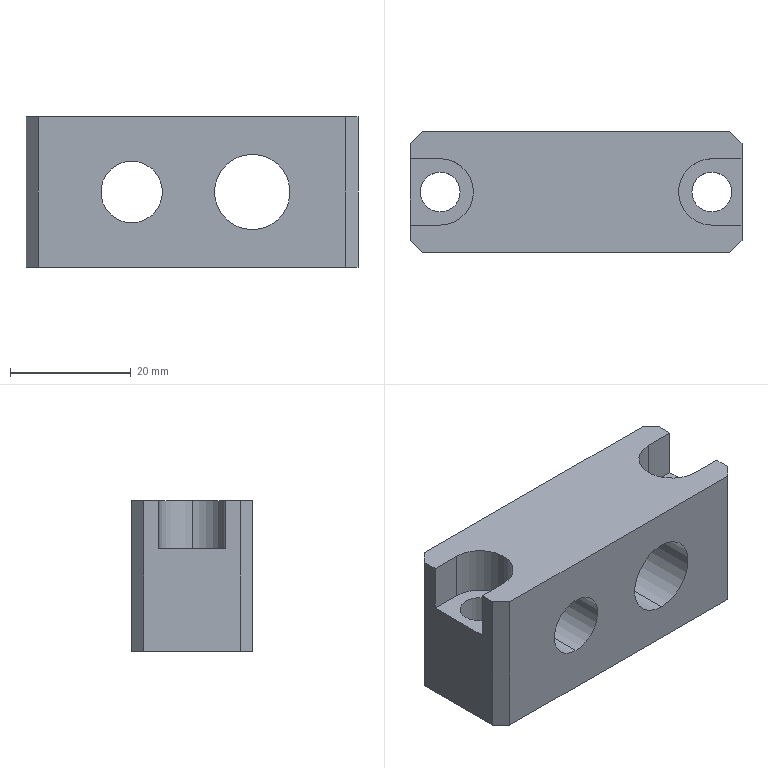Part | SolidWorks | features HoleWzd 3, Chamfer 1, Extrusion 1, ICE 1 | 1 solid | 27 faces | box 55 x 20 x 25 mm | volume 20408 mm3 | plane 16 | cylinder 11 | commonest cylinder face diameters 6.6 x4 11 x3 10.2 x2 12.5 x2
STEP:
#1=CARTESIAN_POINT('',(10.549,13.11,18.75));
#2=VERTEX_POINT('',#1);
#3=CARTESIAN_POINT('',(10.549,13.11,6.25));
#4=VERTEX_POINT('',#3);
#5=CARTESIAN_POINT('',(10.549,13.11,12.5));
#6=DIRECTION('',(0.,-1.,0.));
#7=DIRECTION('',(0.,0.,-1.));
#8=AXIS2_PLACEMENT_3D('',#5,#6,#7);
#9=CIRCLE('',#8,6.25);
#10=EDGE_CURVE('',#2,#4,#9,.T.);
#11=ORIENTED_EDGE('',*,*,#10,.F.);
#12=CARTESIAN_POINT('',(10.549,-6.89,18.75));
#13=VERTEX_POINT('',#12);
#14=CARTESIAN_POINT('',(10.549,-6.89,18.75));
#15=DIRECTION('',(0.,-1.,0.));
#16=VECTOR('',#15,1000.);
#17=LINE('',#14,#16);
#18=EDGE_CURVE('',#2,#13,#17,.T.);
#19=ORIENTED_EDGE('',*,*,#18,.T.);
#20=CARTESIAN_POINT('',(10.549,-6.89,6.25));
#21=VERTEX_POINT('',#20);
#22=CARTESIAN_POINT('',(10.549,-6.89,12.5));
#23=DIRECTION('',(0.,-1.,0.));
#24=DIRECTION('',(0.,0.,-1.));
#25=AXIS2_PLACEMENT_3D('',#22,#23,#24);
#26=CIRCLE('',#25,6.25);
#27=EDGE_CURVE('',#13,#21,#26,.T.);
#28=ORIENTED_EDGE('',*,*,#27,.T.);
#29=CARTESIAN_POINT('',(10.549,-6.89,6.25));
#30=DIRECTION('',(0.,-1.,0.));
#31=VECTOR('',#30,1000.);
#32=LINE('',#29,#31);
#33=EDGE_CURVE('',#4,#21,#32,.T.);
#34=ORIENTED_EDGE('',*,*,#33,.F.);
#35=EDGE_LOOP('',(#11,#19,#28,#34));
#36=FACE_OUTER_BOUND('',#35,.T.);
#37=CARTESIAN_POINT('',(10.549,-6.89,12.5));
#38=DIRECTION('',(0.,-1.,0.));
#39=DIRECTION('',(0.,0.,-1.));
#40=AXIS2_PLACEMENT_3D('',#37,#38,#39);
#41=CYLINDRICAL_SURFACE('',#40,6.25);
#42=ADVANCED_FACE('',(#36),#41,.F.);
#43=CARTESIAN_POINT('',(-9.451,13.11,17.6));
#44=VERTEX_POINT('',#43);
#45=CARTESIAN_POINT('',(-9.451,13.11,7.4));
#46=VERTEX_POINT('',#45);
#47=CARTESIAN_POINT('',(-9.451,13.11,12.5));
#48=DIRECTION('',(0.,-1.,0.));
#49=DIRECTION('',(0.,0.,-1.));
#50=AXIS2_PLACEMENT_3D('',#47,#48,#49);
#51=CIRCLE('',#50,5.1);
#52=EDGE_CURVE('',#44,#46,#51,.T.);
#53=ORIENTED_EDGE('',*,*,#52,.F.);
#54=CARTESIAN_POINT('',(-9.451,-6.89,17.6));
#55=VERTEX_POINT('',#54);
#56=CARTESIAN_POINT('',(-9.451,-6.89,17.6));
#57=DIRECTION('',(0.,-1.,0.));
#58=VECTOR('',#57,1000.);
#59=LINE('',#56,#58);
#60=EDGE_CURVE('',#44,#55,#59,.T.);
#61=ORIENTED_EDGE('',*,*,#60,.T.);
#62=CARTESIAN_POINT('',(-9.451,-6.89,7.4));
#63=VERTEX_POINT('',#62);
#64=CARTESIAN_POINT('',(-9.451,-6.89,12.5));
#65=DIRECTION('',(0.,-1.,0.));
#66=DIRECTION('',(0.,0.,-1.));
#67=AXIS2_PLACEMENT_3D('',#64,#65,#66);
#68=CIRCLE('',#67,5.1);
#69=EDGE_CURVE('',#55,#63,#68,.T.);
#70=ORIENTED_EDGE('',*,*,#69,.T.);
#71=CARTESIAN_POINT('',(-9.451,-6.89,7.4));
#72=DIRECTION('',(0.,-1.,0.));
#73=VECTOR('',#72,1000.);
#74=LINE('',#71,#73);
#75=EDGE_CURVE('',#46,#63,#74,.T.);
#76=ORIENTED_EDGE('',*,*,#75,.F.);
#77=EDGE_LOOP('',(#53,#61,#70,#76));
#78=FACE_OUTER_BOUND('',#77,.T.);
#79=CARTESIAN_POINT('',(-9.451,-6.89,12.5));
#80=DIRECTION('',(0.,-1.,0.));
#81=DIRECTION('',(0.,0.,-1.));
#82=AXIS2_PLACEMENT_3D('',#79,#80,#81);
#83=CYLINDRICAL_SURFACE('',#82,5.1);
#84=ADVANCED_FACE('',(#78),#83,.F.);
#85=CARTESIAN_POINT('',(-25.251,3.11,0.));
#86=VERTEX_POINT('',#85);
#87=CARTESIAN_POINT('',(-18.651,3.11,0.));
#88=VERTEX_POINT('',#87);
#89=CARTESIAN_POINT('',(-21.951,3.11,0.));
#90=DIRECTION('',(0.,0.,1.));
#91=DIRECTION('',(1.,0.,0.));
#92=AXIS2_PLACEMENT_3D('',#89,#90,#91);
#93=CIRCLE('',#92,3.3);
#94=EDGE_CURVE('',#86,#88,#93,.T.);
#95=ORIENTED_EDGE('',*,*,#94,.F.);
#96=CARTESIAN_POINT('',(-25.251,3.11,17.));
#97=VERTEX_POINT('',#96);
#98=CARTESIAN_POINT('',(-25.251,3.11,17.));
#99=DIRECTION('',(0.,0.,1.));
#100=VECTOR('',#99,1000.);
#101=LINE('',#98,#100);
#102=EDGE_CURVE('',#86,#97,#101,.T.);
#103=ORIENTED_EDGE('',*,*,#102,.T.);
#104=CARTESIAN_POINT('',(-18.651,3.11,17.));
#105=VERTEX_POINT('',#104);
#106=CARTESIAN_POINT('',(-21.951,3.11,17.));
#107=DIRECTION('',(0.,0.,1.));
#108=DIRECTION('',(1.,0.,0.));
#109=AXIS2_PLACEMENT_3D('',#106,#107,#108);
#110=CIRCLE('',#109,3.3);
#111=EDGE_CURVE('',#97,#105,#110,.T.);
#112=ORIENTED_EDGE('',*,*,#111,.T.);
#113=CARTESIAN_POINT('',(-18.651,3.11,17.));
#114=DIRECTION('',(0.,0.,1.));
#115=VECTOR('',#114,1000.);
#116=LINE('',#113,#115);
#117=EDGE_CURVE('',#88,#105,#116,.T.);
#118=ORIENTED_EDGE('',*,*,#117,.F.);
#119=EDGE_LOOP('',(#95,#103,#112,#118));
#120=FACE_OUTER_BOUND('',#119,.T.);
#121=CARTESIAN_POINT('',(-21.951,3.11,17.));
#122=DIRECTION('',(0.,0.,1.));
#123=DIRECTION('',(1.,0.,0.));
#124=AXIS2_PLACEMENT_3D('',#121,#122,#123);
#125=CYLINDRICAL_SURFACE('',#124,3.3);
#126=ADVANCED_FACE('',(#120),#125,.F.);
#127=CARTESIAN_POINT('',(19.749,3.11,0.));
#128=VERTEX_POINT('',#127);
#129=CARTESIAN_POINT('',(26.349,3.11,0.));
#130=VERTEX_POINT('',#129);
#131=CARTESIAN_POINT('',(23.049,3.11,0.));
#132=DIRECTION('',(0.,0.,1.));
#133=DIRECTION('',(1.,0.,0.));
#134=AXIS2_PLACEMENT_3D('',#131,#132,#133);
#135=CIRCLE('',#134,3.3);
#136=EDGE_CURVE('',#128,#130,#135,.T.);
#137=ORIENTED_EDGE('',*,*,#136,.F.);
#138=CARTESIAN_POINT('',(19.749,3.11,17.));
#139=VERTEX_POINT('',#138);
#140=CARTESIAN_POINT('',(19.749,3.11,17.));
#141=DIRECTION('',(0.,0.,1.));
#142=VECTOR('',#141,1000.);
#143=LINE('',#140,#142);
#144=EDGE_CURVE('',#128,#139,#143,.T.);
#145=ORIENTED_EDGE('',*,*,#144,.T.);
#146=CARTESIAN_POINT('',(26.349,3.11,17.));
#147=VERTEX_POINT('',#146);
#148=CARTESIAN_POINT('',(23.049,3.11,17.));
#149=DIRECTION('',(0.,0.,1.));
#150=DIRECTION('',(1.,0.,0.));
#151=AXIS2_PLACEMENT_3D('',#148,#149,#150);
#152=CIRCLE('',#151,3.3);
#153=EDGE_CURVE('',#139,#147,#152,.T.);
#154=ORIENTED_EDGE('',*,*,#153,.T.);
#155=CARTESIAN_POINT('',(26.349,3.11,17.));
#156=DIRECTION('',(0.,0.,1.));
#157=VECTOR('',#156,1000.);
#158=LINE('',#155,#157);
#159=EDGE_CURVE('',#130,#147,#158,.T.);
#160=ORIENTED_EDGE('',*,*,#159,.F.);
#161=EDGE_LOOP('',(#137,#145,#154,#160));
#162=FACE_OUTER_BOUND('',#161,.T.);
#163=CARTESIAN_POINT('',(23.049,3.11,17.));
#164=DIRECTION('',(0.,0.,1.));
#165=DIRECTION('',(1.,0.,0.));
#166=AXIS2_PLACEMENT_3D('',#163,#164,#165);
#167=CYLINDRICAL_SURFACE('',#166,3.3);
#168=ADVANCED_FACE('',(#162),#167,.F.);
#169=CARTESIAN_POINT('',(-16.451,3.11,17.));
#170=VERTEX_POINT('',#169);
#171=CARTESIAN_POINT('',(-21.951,8.61,17.));
#172=VERTEX_POINT('',#171);
#173=CARTESIAN_POINT('',(-21.951,3.11,17.));
#174=DIRECTION('',(0.,0.,1.));
#175=DIRECTION('',(1.,0.,0.));
#176=AXIS2_PLACEMENT_3D('',#173,#174,#175);
#177=CIRCLE('',#176,5.5);
#178=EDGE_CURVE('',#170,#172,#177,.T.);
#179=ORIENTED_EDGE('',*,*,#178,.F.);
#180=CARTESIAN_POINT('',(-16.451,3.11,25.));
#181=VERTEX_POINT('',#180);
#182=CARTESIAN_POINT('',(-16.451,3.11,17.));
#183=DIRECTION('',(0.,0.,1.));
#184=VECTOR('',#183,1000.);
#185=LINE('',#182,#184);
#186=EDGE_CURVE('',#170,#181,#185,.T.);
#187=ORIENTED_EDGE('',*,*,#186,.T.);
#188=CARTESIAN_POINT('',(-21.951,8.61,25.));
#189=VERTEX_POINT('',#188);
#190=CARTESIAN_POINT('',(-21.951,3.11,25.));
#191=DIRECTION('',(0.,0.,1.));
#192=DIRECTION('',(1.,0.,0.));
#193=AXIS2_PLACEMENT_3D('',#190,#191,#192);
#194=CIRCLE('',#193,5.5);
#195=EDGE_CURVE('',#181,#189,#194,.T.);
#196=ORIENTED_EDGE('',*,*,#195,.T.);
#197=CARTESIAN_POINT('',(-21.951,8.61,17.));
#198=DIRECTION('',(0.,0.,1.));
#199=VECTOR('',#198,1000.);
#200=LINE('',#197,#199);
#201=EDGE_CURVE('',#172,#189,#200,.T.);
#202=ORIENTED_EDGE('',*,*,#201,.F.);
#203=EDGE_LOOP('',(#179,#187,#196,#202));
#204=FACE_OUTER_BOUND('',#203,.T.);
#205=CARTESIAN_POINT('',(-21.951,3.11,17.));
#206=DIRECTION('',(0.,0.,1.));
#207=DIRECTION('',(1.,0.,0.));
#208=AXIS2_PLACEMENT_3D('',#205,#206,#207);
#209=CYLINDRICAL_SURFACE('',#208,5.5);
#210=ADVANCED_FACE('',(#204),#209,.F.);
#211=CARTESIAN_POINT('',(-26.951,-2.39,25.));
#212=VERTEX_POINT('',#211);
#213=CARTESIAN_POINT('',(-26.951,-4.89,25.));
#214=VERTEX_POINT('',#213);
#215=CARTESIAN_POINT('',(-26.951,13.11,25.));
#216=DIRECTION('',(0.,-1.,0.));
#217=VECTOR('',#216,1000.);
#218=LINE('',#215,#217);
#219=EDGE_CURVE('',#212,#214,#218,.T.);
#220=ORIENTED_EDGE('',*,*,#219,.F.);
#221=CARTESIAN_POINT('',(-26.951,-2.39,17.));
#222=VERTEX_POINT('',#221);
#223=CARTESIAN_POINT('',(-26.951,-2.39,17.));
#224=DIRECTION('',(0.,0.,1.));
#225=VECTOR('',#224,1000.);
#226=LINE('',#223,#225);
#227=EDGE_CURVE('',#222,#212,#226,.T.);
#228=ORIENTED_EDGE('',*,*,#227,.F.);
#229=CARTESIAN_POINT('',(-26.951,8.61,17.));
#230=VERTEX_POINT('',#229);
#231=CARTESIAN_POINT('',(-26.951,8.61,17.));
#232=DIRECTION('',(0.,-1.,0.));
#233=VECTOR('',#232,1000.);
#234=LINE('',#231,#233);
#235=EDGE_CURVE('',#230,#222,#234,.T.);
#236=ORIENTED_EDGE('',*,*,#235,.F.);
#237=CARTESIAN_POINT('',(-26.951,8.61,25.));
#238=VERTEX_POINT('',#237);
#239=CARTESIAN_POINT('',(-26.951,8.61,17.));
#240=DIRECTION('',(0.,0.,1.));
#241=VECTOR('',#240,1000.);
#242=LINE('',#239,#241);
#243=EDGE_CURVE('',#230,#238,#242,.T.);
#244=ORIENTED_EDGE('',*,*,#243,.T.);
#245=CARTESIAN_POINT('',(-26.951,11.11,25.));
#246=VERTEX_POINT('',#245);
#247=CARTESIAN_POINT('',(-26.951,13.11,25.));
#248=DIRECTION('',(0.,-1.,0.));
#249=VECTOR('',#248,1000.);
#250=LINE('',#247,#249);
#251=EDGE_CURVE('',#246,#238,#250,.T.);
#252=ORIENTED_EDGE('',*,*,#251,.F.);
#253=CARTESIAN_POINT('',(-26.951,11.11,0.));
#254=VERTEX_POINT('',#253);
#255=CARTESIAN_POINT('',(-26.951,11.11,25.));
#256=DIRECTION('',(0.,0.,-1.));
#257=VECTOR('',#256,1000.);
#258=LINE('',#255,#257);
#259=EDGE_CURVE('',#246,#254,#258,.T.);
#260=ORIENTED_EDGE('',*,*,#259,.T.);
#261=CARTESIAN_POINT('',(-26.951,-4.89,0.));
#262=VERTEX_POINT('',#261);
#263=CARTESIAN_POINT('',(-26.951,13.11,0.));
#264=DIRECTION('',(0.,-1.,0.));
#265=VECTOR('',#264,1000.);
#266=LINE('',#263,#265);
#267=EDGE_CURVE('',#254,#262,#266,.T.);
#268=ORIENTED_EDGE('',*,*,#267,.T.);
#269=CARTESIAN_POINT('',(-26.951,-4.89,25.));
#270=DIRECTION('',(0.,0.,1.));
#271=VECTOR('',#270,1000.);
#272=LINE('',#269,#271);
#273=EDGE_CURVE('',#262,#214,#272,.T.);
#274=ORIENTED_EDGE('',*,*,#273,.T.);
#275=EDGE_LOOP('',(#220,#228,#236,#244,#252,#260,#268,#274));
#276=FACE_OUTER_BOUND('',#275,.T.);
#277=CARTESIAN_POINT('',(-26.951,13.11,25.));
#278=DIRECTION('',(1.,0.,0.));
#279=DIRECTION('',(0.,1.,0.));
#280=AXIS2_PLACEMENT_3D('',#277,#278,#279);
#281=PLANE('',#280);
#282=ADVANCED_FACE('',(#276),#281,.F.);
#283=CARTESIAN_POINT('',(10.549,-6.89,12.5));
#284=DIRECTION('',(0.,-1.,0.));
#285=DIRECTION('',(0.,0.,-1.));
#286=AXIS2_PLACEMENT_3D('',#283,#284,#285);
#287=CIRCLE('',#286,6.25);
#288=EDGE_CURVE('',#21,#13,#287,.T.);
#289=ORIENTED_EDGE('',*,*,#288,.F.);
#290=ORIENTED_EDGE('',*,*,#27,.F.);
#291=EDGE_LOOP('',(#289,#290));
#292=FACE_BOUND('',#291,.T.);
#293=CARTESIAN_POINT('',(-9.451,-6.89,12.5));
#294=DIRECTION('',(0.,-1.,0.));
#295=DIRECTION('',(0.,0.,-1.));
#296=AXIS2_PLACEMENT_3D('',#293,#294,#295);
#297=CIRCLE('',#296,5.1);
#298=EDGE_CURVE('',#63,#55,#297,.T.);
#299=ORIENTED_EDGE('',*,*,#298,.F.);
#300=ORIENTED_EDGE('',*,*,#69,.F.);
#301=EDGE_LOOP('',(#299,#300));
#302=FACE_BOUND('',#301,.T.);
#303=CARTESIAN_POINT('',(-24.951,-6.89,0.));
#304=VERTEX_POINT('',#303);
#305=CARTESIAN_POINT('',(26.049,-6.89,0.));
#306=VERTEX_POINT('',#305);
#307=CARTESIAN_POINT('',(-26.951,-6.89,0.));
#308=DIRECTION('',(1.,0.,0.));
#309=VECTOR('',#308,1000.);
#310=LINE('',#307,#309);
#311=EDGE_CURVE('',#304,#306,#310,.T.);
#312=ORIENTED_EDGE('',*,*,#311,.T.);
#313=CARTESIAN_POINT('',(26.049,-6.89,25.));
#314=VERTEX_POINT('',#313);
#315=CARTESIAN_POINT('',(26.049,-6.89,25.));
#316=DIRECTION('',(0.,0.,1.));
#317=VECTOR('',#316,1000.);
#318=LINE('',#315,#317);
#319=EDGE_CURVE('',#306,#314,#318,.T.);
#320=ORIENTED_EDGE('',*,*,#319,.T.);
#321=CARTESIAN_POINT('',(-24.951,-6.89,25.));
#322=VERTEX_POINT('',#321);
#323=CARTESIAN_POINT('',(-26.951,-6.89,25.));
#324=DIRECTION('',(1.,0.,0.));
#325=VECTOR('',#324,1000.);
#326=LINE('',#323,#325);
#327=EDGE_CURVE('',#322,#314,#326,.T.);
#328=ORIENTED_EDGE('',*,*,#327,.F.);
#329=CARTESIAN_POINT('',(-24.951,-6.89,25.));
#330=DIRECTION('',(0.,0.,-1.));
#331=VECTOR('',#330,1000.);
#332=LINE('',#329,#331);
#333=EDGE_CURVE('',#322,#304,#332,.T.);
#334=ORIENTED_EDGE('',*,*,#333,.T.);
#335=EDGE_LOOP('',(#312,#320,#328,#334));
#336=FACE_OUTER_BOUND('',#335,.T.);
#337=CARTESIAN_POINT('',(-26.951,-6.89,25.));
#338=DIRECTION('',(0.,1.,0.));
#339=DIRECTION('',(0.,0.,1.));
#340=AXIS2_PLACEMENT_3D('',#337,#338,#339);
#341=PLANE('',#340);
#342=ADVANCED_FACE('',(#292,#302,#336),#341,.F.);
#343=CARTESIAN_POINT('',(28.049,8.61,25.));
#344=VERTEX_POINT('',#343);
#345=CARTESIAN_POINT('',(28.049,11.11,25.));
#346=VERTEX_POINT('',#345);
#347=CARTESIAN_POINT('',(28.049,13.11,25.));
#348=DIRECTION('',(0.,1.,0.));
#349=VECTOR('',#348,1000.);
#350=LINE('',#347,#349);
#351=EDGE_CURVE('',#344,#346,#350,.T.);
#352=ORIENTED_EDGE('',*,*,#351,.F.);
#353=CARTESIAN_POINT('',(28.049,8.61,17.));
#354=VERTEX_POINT('',#353);
#355=CARTESIAN_POINT('',(28.049,8.61,17.));
#356=DIRECTION('',(0.,0.,1.));
#357=VECTOR('',#356,1000.);
#358=LINE('',#355,#357);
#359=EDGE_CURVE('',#354,#344,#358,.T.);
#360=ORIENTED_EDGE('',*,*,#359,.F.);
#361=CARTESIAN_POINT('',(28.049,-2.39,17.));
#362=VERTEX_POINT('',#361);
#363=CARTESIAN_POINT('',(28.049,8.61,17.));
#364=DIRECTION('',(0.,1.,0.));
#365=VECTOR('',#364,1000.);
#366=LINE('',#363,#365);
#367=EDGE_CURVE('',#362,#354,#366,.T.);
#368=ORIENTED_EDGE('',*,*,#367,.F.);
#369=CARTESIAN_POINT('',(28.049,-2.39,25.));
#370=VERTEX_POINT('',#369);
#371=CARTESIAN_POINT('',(28.049,-2.39,17.));
#372=DIRECTION('',(0.,0.,1.));
#373=VECTOR('',#372,1000.);
#374=LINE('',#371,#373);
#375=EDGE_CURVE('',#362,#370,#374,.T.);
#376=ORIENTED_EDGE('',*,*,#375,.T.);
#377=CARTESIAN_POINT('',(28.049,-4.89,25.));
#378=VERTEX_POINT('',#377);
#379=CARTESIAN_POINT('',(28.049,13.11,25.));
#380=DIRECTION('',(0.,1.,0.));
#381=VECTOR('',#380,1000.);
#382=LINE('',#379,#381);
#383=EDGE_CURVE('',#378,#370,#382,.T.);
#384=ORIENTED_EDGE('',*,*,#383,.F.);
#385=CARTESIAN_POINT('',(28.049,-4.89,0.));
#386=VERTEX_POINT('',#385);
#387=CARTESIAN_POINT('',(28.049,-4.89,25.));
#388=DIRECTION('',(0.,0.,-1.));
#389=VECTOR('',#388,1000.);
#390=LINE('',#387,#389);
#391=EDGE_CURVE('',#378,#386,#390,.T.);
#392=ORIENTED_EDGE('',*,*,#391,.T.);
#393=CARTESIAN_POINT('',(28.049,11.11,0.));
#394=VERTEX_POINT('',#393);
#395=CARTESIAN_POINT('',(28.049,13.11,0.));
#396=DIRECTION('',(0.,1.,0.));
#397=VECTOR('',#396,1000.);
#398=LINE('',#395,#397);
#399=EDGE_CURVE('',#386,#394,#398,.T.);
#400=ORIENTED_EDGE('',*,*,#399,.T.);
#401=CARTESIAN_POINT('',(28.049,11.11,25.));
#402=DIRECTION('',(0.,0.,1.));
#403=VECTOR('',#402,1000.);
#404=LINE('',#401,#403);
#405=EDGE_CURVE('',#394,#346,#404,.T.);
#406=ORIENTED_EDGE('',*,*,#405,.T.);
#407=EDGE_LOOP('',(#352,#360,#368,#376,#384,#392,#400,#406));
#408=FACE_OUTER_BOUND('',#407,.T.);
#409=CARTESIAN_POINT('',(28.049,13.11,25.));
#410=DIRECTION('',(-1.,0.,0.));
#411=DIRECTION('',(0.,-1.,0.));
#412=AXIS2_PLACEMENT_3D('',#409,#410,#411);
#413=PLANE('',#412);
#414=ADVANCED_FACE('',(#408),#413,.F.);
#415=CARTESIAN_POINT('',(10.549,13.11,12.5));
#416=DIRECTION('',(0.,-1.,0.));
#417=DIRECTION('',(0.,0.,-1.));
#418=AXIS2_PLACEMENT_3D('',#415,#416,#417);
#419=CIRCLE('',#418,6.25);
#420=EDGE_CURVE('',#4,#2,#419,.T.);
#421=ORIENTED_EDGE('',*,*,#420,.T.);
#422=ORIENTED_EDGE('',*,*,#10,.T.);
#423=EDGE_LOOP('',(#421,#422));
#424=FACE_BOUND('',#423,.T.);
#425=CARTESIAN_POINT('',(-9.451,13.11,12.5));
#426=DIRECTION('',(0.,-1.,0.));
#427=DIRECTION('',(0.,0.,-1.));
#428=AXIS2_PLACEMENT_3D('',#425,#426,#427);
#429=CIRCLE('',#428,5.1);
#430=EDGE_CURVE('',#46,#44,#429,.T.);
#431=ORIENTED_EDGE('',*,*,#430,.T.);
#432=ORIENTED_EDGE('',*,*,#52,.T.);
#433=EDGE_LOOP('',(#431,#432));
#434=FACE_BOUND('',#433,.T.);
#435=CARTESIAN_POINT('',(26.049,13.11,25.));
#436=VERTEX_POINT('',#435);
#437=CARTESIAN_POINT('',(-24.951,13.11,25.));
#438=VERTEX_POINT('',#437);
#439=CARTESIAN_POINT('',(-26.951,13.11,25.));
#440=DIRECTION('',(-1.,0.,0.));
#441=VECTOR('',#440,1000.);
#442=LINE('',#439,#441);
#443=EDGE_CURVE('',#436,#438,#442,.T.);
#444=ORIENTED_EDGE('',*,*,#443,.F.);
#445=CARTESIAN_POINT('',(26.049,13.11,0.));
#446=VERTEX_POINT('',#445);
#447=CARTESIAN_POINT('',(26.049,13.11,25.));
#448=DIRECTION('',(0.,0.,-1.));
#449=VECTOR('',#448,1000.);
#450=LINE('',#447,#449);
#451=EDGE_CURVE('',#436,#446,#450,.T.);
#452=ORIENTED_EDGE('',*,*,#451,.T.);
#453=CARTESIAN_POINT('',(-24.951,13.11,0.));
#454=VERTEX_POINT('',#453);
#455=CARTESIAN_POINT('',(-26.951,13.11,0.));
#456=DIRECTION('',(-1.,0.,0.));
#457=VECTOR('',#456,1000.);
#458=LINE('',#455,#457);
#459=EDGE_CURVE('',#446,#454,#458,.T.);
#460=ORIENTED_EDGE('',*,*,#459,.T.);
#461=CARTESIAN_POINT('',(-24.951,13.11,25.));
#462=DIRECTION('',(0.,0.,1.));
#463=VECTOR('',#462,1000.);
#464=LINE('',#461,#463);
#465=EDGE_CURVE('',#454,#438,#464,.T.);
#466=ORIENTED_EDGE('',*,*,#465,.T.);
#467=EDGE_LOOP('',(#444,#452,#460,#466));
#468=FACE_OUTER_BOUND('',#467,.T.);
#469=CARTESIAN_POINT('',(-26.951,13.11,25.));
#470=DIRECTION('',(0.,-1.,0.));
#471=DIRECTION('',(0.,0.,-1.));
#472=AXIS2_PLACEMENT_3D('',#469,#470,#471);
#473=PLANE('',#472);
#474=ADVANCED_FACE('',(#424,#434,#468),#473,.F.);
#475=CARTESIAN_POINT('',(-21.951,-2.39,25.));
#476=VERTEX_POINT('',#475);
#477=CARTESIAN_POINT('',(-26.951,-2.39,25.));
#478=DIRECTION('',(1.,0.,0.));
#479=VECTOR('',#478,1000.);
#480=LINE('',#477,#479);
#481=EDGE_CURVE('',#212,#476,#480,.T.);
#482=ORIENTED_EDGE('',*,*,#481,.F.);
#483=ORIENTED_EDGE('',*,*,#219,.T.);
#484=CARTESIAN_POINT('',(-15.92,-15.92,25.));
#485=DIRECTION('',(0.7071,-0.7071,0.));
#486=VECTOR('',#485,1000.);
#487=LINE('',#484,#486);
#488=EDGE_CURVE('',#214,#322,#487,.T.);
#489=ORIENTED_EDGE('',*,*,#488,.T.);
#490=ORIENTED_EDGE('',*,*,#327,.T.);
#491=CARTESIAN_POINT('',(16.469,-16.469,25.));
#492=DIRECTION('',(0.7071,0.7071,0.));
#493=VECTOR('',#492,1000.);
#494=LINE('',#491,#493);
#495=EDGE_CURVE('',#314,#378,#494,.T.);
#496=ORIENTED_EDGE('',*,*,#495,.T.);
#497=ORIENTED_EDGE('',*,*,#383,.T.);
#498=CARTESIAN_POINT('',(23.049,-2.39,25.));
#499=VERTEX_POINT('',#498);
#500=CARTESIAN_POINT('',(28.049,-2.39,25.));
#501=DIRECTION('',(1.,0.,0.));
#502=VECTOR('',#501,1000.);
#503=LINE('',#500,#502);
#504=EDGE_CURVE('',#499,#370,#503,.T.);
#505=ORIENTED_EDGE('',*,*,#504,.F.);
#506=CARTESIAN_POINT('',(23.049,8.61,25.));
#507=VERTEX_POINT('',#506);
#508=CARTESIAN_POINT('',(23.049,3.11,25.));
#509=DIRECTION('',(0.,0.,1.));
#510=DIRECTION('',(1.,0.,0.));
#511=AXIS2_PLACEMENT_3D('',#508,#509,#510);
#512=CIRCLE('',#511,5.5);
#513=EDGE_CURVE('',#507,#499,#512,.T.);
#514=ORIENTED_EDGE('',*,*,#513,.F.);
#515=CARTESIAN_POINT('',(23.049,8.61,25.));
#516=DIRECTION('',(-1.,0.,0.));
#517=VECTOR('',#516,1000.);
#518=LINE('',#515,#517);
#519=EDGE_CURVE('',#344,#507,#518,.T.);
#520=ORIENTED_EDGE('',*,*,#519,.F.);
#521=ORIENTED_EDGE('',*,*,#351,.T.);
#522=CARTESIAN_POINT('',(19.58,19.58,25.));
#523=DIRECTION('',(-0.7071,0.7071,0.));
#524=VECTOR('',#523,1000.);
#525=LINE('',#522,#524);
#526=EDGE_CURVE('',#346,#436,#525,.T.);
#527=ORIENTED_EDGE('',*,*,#526,.T.);
#528=ORIENTED_EDGE('',*,*,#443,.T.);
#529=CARTESIAN_POINT('',(-19.031,19.031,25.));
#530=DIRECTION('',(-0.7071,-0.7071,0.));
#531=VECTOR('',#530,1000.);
#532=LINE('',#529,#531);
#533=EDGE_CURVE('',#438,#246,#532,.T.);
#534=ORIENTED_EDGE('',*,*,#533,.T.);
#535=ORIENTED_EDGE('',*,*,#251,.T.);
#536=CARTESIAN_POINT('',(-21.951,8.61,25.));
#537=DIRECTION('',(-1.,0.,0.));
#538=VECTOR('',#537,1000.);
#539=LINE('',#536,#538);
#540=EDGE_CURVE('',#189,#238,#539,.T.);
#541=ORIENTED_EDGE('',*,*,#540,.F.);
#542=ORIENTED_EDGE('',*,*,#195,.F.);
#543=CARTESIAN_POINT('',(-21.951,3.11,25.));
#544=DIRECTION('',(0.,0.,1.));
#545=DIRECTION('',(1.,0.,0.));
#546=AXIS2_PLACEMENT_3D('',#543,#544,#545);
#547=CIRCLE('',#546,5.5);
#548=EDGE_CURVE('',#476,#181,#547,.T.);
#549=ORIENTED_EDGE('',*,*,#548,.F.);
#550=EDGE_LOOP('',(#482,#483,#489,#490,#496,#497,#505,#514,#520,#521,#527,#528,#534,#535,#541,#542,#549));
#551=FACE_OUTER_BOUND('',#550,.T.);
#552=CARTESIAN_POINT('',(0.,0.,25.));
#553=DIRECTION('',(0.,0.,1.));
#554=DIRECTION('',(1.,0.,0.));
#555=AXIS2_PLACEMENT_3D('',#552,#553,#554);
#556=PLANE('',#555);
#557=ADVANCED_FACE('',(#551),#556,.T.);
#558=CARTESIAN_POINT('',(-21.951,3.11,0.));
#559=DIRECTION('',(0.,0.,1.));
#560=DIRECTION('',(1.,0.,0.));
#561=AXIS2_PLACEMENT_3D('',#558,#559,#560);
#562=CIRCLE('',#561,3.3);
#563=EDGE_CURVE('',#88,#86,#562,.T.);
#564=ORIENTED_EDGE('',*,*,#563,.T.);
#565=ORIENTED_EDGE('',*,*,#94,.T.);
#566=EDGE_LOOP('',(#564,#565));
#567=FACE_BOUND('',#566,.T.);
#568=CARTESIAN_POINT('',(23.049,3.11,0.));
#569=DIRECTION('',(0.,0.,1.));
#570=DIRECTION('',(1.,0.,0.));
#571=AXIS2_PLACEMENT_3D('',#568,#569,#570);
#572=CIRCLE('',#571,3.3);
#573=EDGE_CURVE('',#130,#128,#572,.T.);
#574=ORIENTED_EDGE('',*,*,#573,.T.);
#575=ORIENTED_EDGE('',*,*,#136,.T.);
#576=EDGE_LOOP('',(#574,#575));
#577=FACE_BOUND('',#576,.T.);
#578=ORIENTED_EDGE('',*,*,#459,.F.);
#579=CARTESIAN_POINT('',(26.049,13.11,0.));
#580=DIRECTION('',(0.7071,-0.7071,0.));
#581=VECTOR('',#580,1000.);
#582=LINE('',#579,#581);
#583=EDGE_CURVE('',#446,#394,#582,.T.);
#584=ORIENTED_EDGE('',*,*,#583,.T.);
#585=ORIENTED_EDGE('',*,*,#399,.F.);
#586=CARTESIAN_POINT('',(28.049,-4.89,0.));
#587=DIRECTION('',(-0.7071,-0.7071,0.));
#588=VECTOR('',#587,1000.);
#589=LINE('',#586,#588);
#590=EDGE_CURVE('',#386,#306,#589,.T.);
#591=ORIENTED_EDGE('',*,*,#590,.T.);
#592=ORIENTED_EDGE('',*,*,#311,.F.);
#593=CARTESIAN_POINT('',(-24.951,-6.89,0.));
#594=DIRECTION('',(-0.7071,0.7071,0.));
#595=VECTOR('',#594,1000.);
#596=LINE('',#593,#595);
#597=EDGE_CURVE('',#304,#262,#596,.T.);
#598=ORIENTED_EDGE('',*,*,#597,.T.);
#599=ORIENTED_EDGE('',*,*,#267,.F.);
#600=CARTESIAN_POINT('',(-26.951,11.11,0.));
#601=DIRECTION('',(0.7071,0.7071,0.));
#602=VECTOR('',#601,1000.);
#603=LINE('',#600,#602);
#604=EDGE_CURVE('',#254,#454,#603,.T.);
#605=ORIENTED_EDGE('',*,*,#604,.T.);
#606=EDGE_LOOP('',(#578,#584,#585,#591,#592,#598,#599,#605));
#607=FACE_OUTER_BOUND('',#606,.T.);
#608=CARTESIAN_POINT('',(0.,0.,0.));
#609=DIRECTION('',(0.,0.,1.));
#610=DIRECTION('',(1.,0.,0.));
#611=AXIS2_PLACEMENT_3D('',#608,#609,#610);
#612=PLANE('',#611);
#613=ADVANCED_FACE('',(#567,#577,#607),#612,.F.);
#614=ORIENTED_EDGE('',*,*,#526,.F.);
#615=ORIENTED_EDGE('',*,*,#405,.F.);
#616=ORIENTED_EDGE('',*,*,#583,.F.);
#617=ORIENTED_EDGE('',*,*,#451,.F.);
#618=EDGE_LOOP('',(#614,#615,#616,#617));
#619=FACE_OUTER_BOUND('',#618,.T.);
#620=CARTESIAN_POINT('',(26.049,13.11,25.));
#621=DIRECTION('',(-0.7071,-0.7071,0.));
#622=DIRECTION('',(0.,0.,-1.));
#623=AXIS2_PLACEMENT_3D('',#620,#621,#622);
#624=PLANE('',#623);
#625=ADVANCED_FACE('',(#619),#624,.F.);
#626=ORIENTED_EDGE('',*,*,#495,.F.);
#627=ORIENTED_EDGE('',*,*,#319,.F.);
#628=ORIENTED_EDGE('',*,*,#590,.F.);
#629=ORIENTED_EDGE('',*,*,#391,.F.);
#630=EDGE_LOOP('',(#626,#627,#628,#629));
#631=FACE_OUTER_BOUND('',#630,.T.);
#632=CARTESIAN_POINT('',(28.049,-4.89,25.));
#633=DIRECTION('',(-0.7071,0.7071,0.));
#634=DIRECTION('',(0.,0.,-1.));
#635=AXIS2_PLACEMENT_3D('',#632,#633,#634);
#636=PLANE('',#635);
#637=ADVANCED_FACE('',(#631),#636,.F.);
#638=ORIENTED_EDGE('',*,*,#488,.F.);
#639=ORIENTED_EDGE('',*,*,#273,.F.);
#640=ORIENTED_EDGE('',*,*,#597,.F.);
#641=ORIENTED_EDGE('',*,*,#333,.F.);
#642=EDGE_LOOP('',(#638,#639,#640,#641));
#643=FACE_OUTER_BOUND('',#642,.T.);
#644=CARTESIAN_POINT('',(-24.951,-6.89,25.));
#645=DIRECTION('',(0.7071,0.7071,0.));
#646=DIRECTION('',(0.,0.,-1.));
#647=AXIS2_PLACEMENT_3D('',#644,#645,#646);
#648=PLANE('',#647);
#649=ADVANCED_FACE('',(#643),#648,.F.);
#650=ORIENTED_EDGE('',*,*,#533,.F.);
#651=ORIENTED_EDGE('',*,*,#465,.F.);
#652=ORIENTED_EDGE('',*,*,#604,.F.);
#653=ORIENTED_EDGE('',*,*,#259,.F.);
#654=EDGE_LOOP('',(#650,#651,#652,#653));
#655=FACE_OUTER_BOUND('',#654,.T.);
#656=CARTESIAN_POINT('',(-26.951,11.11,25.));
#657=DIRECTION('',(0.7071,-0.7071,0.));
#658=DIRECTION('',(0.,0.,-1.));
#659=AXIS2_PLACEMENT_3D('',#656,#657,#658);
#660=PLANE('',#659);
#661=ADVANCED_FACE('',(#655),#660,.F.);
#662=ORIENTED_EDGE('',*,*,#513,.T.);
#663=CARTESIAN_POINT('',(23.049,-2.39,17.));
#664=VERTEX_POINT('',#663);
#665=CARTESIAN_POINT('',(23.049,-2.39,17.));
#666=DIRECTION('',(0.,0.,1.));
#667=VECTOR('',#666,1000.);
#668=LINE('',#665,#667);
#669=EDGE_CURVE('',#664,#499,#668,.T.);
#670=ORIENTED_EDGE('',*,*,#669,.F.);
#671=CARTESIAN_POINT('',(23.049,8.61,17.));
#672=VERTEX_POINT('',#671);
#673=CARTESIAN_POINT('',(23.049,3.11,17.));
#674=DIRECTION('',(0.,0.,1.));
#675=DIRECTION('',(1.,0.,0.));
#676=AXIS2_PLACEMENT_3D('',#673,#674,#675);
#677=CIRCLE('',#676,5.5);
#678=EDGE_CURVE('',#672,#664,#677,.T.);
#679=ORIENTED_EDGE('',*,*,#678,.F.);
#680=CARTESIAN_POINT('',(23.049,8.61,17.));
#681=DIRECTION('',(0.,0.,1.));
#682=VECTOR('',#681,1000.);
#683=LINE('',#680,#682);
#684=EDGE_CURVE('',#672,#507,#683,.T.);
#685=ORIENTED_EDGE('',*,*,#684,.T.);
#686=EDGE_LOOP('',(#662,#670,#679,#685));
#687=FACE_OUTER_BOUND('',#686,.T.);
#688=CARTESIAN_POINT('',(23.049,3.11,17.));
#689=DIRECTION('',(0.,0.,1.));
#690=DIRECTION('',(1.,0.,0.));
#691=AXIS2_PLACEMENT_3D('',#688,#689,#690);
#692=CYLINDRICAL_SURFACE('',#691,5.5);
#693=ADVANCED_FACE('',(#687),#692,.F.);
#694=ORIENTED_EDGE('',*,*,#519,.T.);
#695=ORIENTED_EDGE('',*,*,#684,.F.);
#696=CARTESIAN_POINT('',(23.049,8.61,17.));
#697=DIRECTION('',(-1.,0.,0.));
#698=VECTOR('',#697,1000.);
#699=LINE('',#696,#698);
#700=EDGE_CURVE('',#354,#672,#699,.T.);
#701=ORIENTED_EDGE('',*,*,#700,.F.);
#702=ORIENTED_EDGE('',*,*,#359,.T.);
#703=EDGE_LOOP('',(#694,#695,#701,#702));
#704=FACE_OUTER_BOUND('',#703,.T.);
#705=CARTESIAN_POINT('',(23.049,8.61,17.));
#706=DIRECTION('',(0.,1.,0.));
#707=DIRECTION('',(-1.,0.,0.));
#708=AXIS2_PLACEMENT_3D('',#705,#706,#707);
#709=PLANE('',#708);
#710=ADVANCED_FACE('',(#704),#709,.F.);
#711=ORIENTED_EDGE('',*,*,#504,.T.);
#712=ORIENTED_EDGE('',*,*,#375,.F.);
#713=CARTESIAN_POINT('',(28.049,-2.39,17.));
#714=DIRECTION('',(1.,0.,0.));
#715=VECTOR('',#714,1000.);
#716=LINE('',#713,#715);
#717=EDGE_CURVE('',#664,#362,#716,.T.);
#718=ORIENTED_EDGE('',*,*,#717,.F.);
#719=ORIENTED_EDGE('',*,*,#669,.T.);
#720=EDGE_LOOP('',(#711,#712,#718,#719));
#721=FACE_OUTER_BOUND('',#720,.T.);
#722=CARTESIAN_POINT('',(28.049,-2.39,17.));
#723=DIRECTION('',(0.,-1.,0.));
#724=DIRECTION('',(0.,0.,-1.));
#725=AXIS2_PLACEMENT_3D('',#722,#723,#724);
#726=PLANE('',#725);
#727=ADVANCED_FACE('',(#721),#726,.F.);
#728=CARTESIAN_POINT('',(23.049,3.11,17.));
#729=DIRECTION('',(0.,0.,1.));
#730=DIRECTION('',(1.,0.,0.));
#731=AXIS2_PLACEMENT_3D('',#728,#729,#730);
#732=CIRCLE('',#731,3.3);
#733=EDGE_CURVE('',#147,#139,#732,.T.);
#734=ORIENTED_EDGE('',*,*,#733,.F.);
#735=ORIENTED_EDGE('',*,*,#153,.F.);
#736=EDGE_LOOP('',(#734,#735));
#737=FACE_BOUND('',#736,.T.);
#738=ORIENTED_EDGE('',*,*,#678,.T.);
#739=ORIENTED_EDGE('',*,*,#717,.T.);
#740=ORIENTED_EDGE('',*,*,#367,.T.);
#741=ORIENTED_EDGE('',*,*,#700,.T.);
#742=EDGE_LOOP('',(#738,#739,#740,#741));
#743=FACE_OUTER_BOUND('',#742,.T.);
#744=CARTESIAN_POINT('',(23.049,3.11,17.));
#745=DIRECTION('',(0.,0.,1.));
#746=DIRECTION('',(1.,0.,0.));
#747=AXIS2_PLACEMENT_3D('',#744,#745,#746);
#748=PLANE('',#747);
#749=ADVANCED_FACE('',(#737,#743),#748,.T.);
#750=ORIENTED_EDGE('',*,*,#186,.F.);
#751=CARTESIAN_POINT('',(-21.951,-2.39,17.));
#752=VERTEX_POINT('',#751);
#753=CARTESIAN_POINT('',(-21.951,3.11,17.));
#754=DIRECTION('',(0.,0.,1.));
#755=DIRECTION('',(1.,0.,0.));
#756=AXIS2_PLACEMENT_3D('',#753,#754,#755);
#757=CIRCLE('',#756,5.5);
#758=EDGE_CURVE('',#752,#170,#757,.T.);
#759=ORIENTED_EDGE('',*,*,#758,.F.);
#760=CARTESIAN_POINT('',(-21.951,-2.39,17.));
#761=DIRECTION('',(0.,0.,1.));
#762=VECTOR('',#761,1000.);
#763=LINE('',#760,#762);
#764=EDGE_CURVE('',#752,#476,#763,.T.);
#765=ORIENTED_EDGE('',*,*,#764,.T.);
#766=ORIENTED_EDGE('',*,*,#548,.T.);
#767=EDGE_LOOP('',(#750,#759,#765,#766));
#768=FACE_OUTER_BOUND('',#767,.T.);
#769=CARTESIAN_POINT('',(-21.951,3.11,17.));
#770=DIRECTION('',(0.,0.,1.));
#771=DIRECTION('',(1.,0.,0.));
#772=AXIS2_PLACEMENT_3D('',#769,#770,#771);
#773=CYLINDRICAL_SURFACE('',#772,5.5);
#774=ADVANCED_FACE('',(#768),#773,.F.);
#775=ORIENTED_EDGE('',*,*,#481,.T.);
#776=ORIENTED_EDGE('',*,*,#764,.F.);
#777=CARTESIAN_POINT('',(-26.951,-2.39,17.));
#778=DIRECTION('',(1.,0.,0.));
#779=VECTOR('',#778,1000.);
#780=LINE('',#777,#779);
#781=EDGE_CURVE('',#222,#752,#780,.T.);
#782=ORIENTED_EDGE('',*,*,#781,.F.);
#783=ORIENTED_EDGE('',*,*,#227,.T.);
#784=EDGE_LOOP('',(#775,#776,#782,#783));
#785=FACE_OUTER_BOUND('',#784,.T.);
#786=CARTESIAN_POINT('',(-26.951,-2.39,17.));
#787=DIRECTION('',(0.,-1.,0.));
#788=DIRECTION('',(0.,0.,-1.));
#789=AXIS2_PLACEMENT_3D('',#786,#787,#788);
#790=PLANE('',#789);
#791=ADVANCED_FACE('',(#785),#790,.F.);
#792=ORIENTED_EDGE('',*,*,#540,.T.);
#793=ORIENTED_EDGE('',*,*,#243,.F.);
#794=CARTESIAN_POINT('',(-21.951,8.61,17.));
#795=DIRECTION('',(-1.,0.,0.));
#796=VECTOR('',#795,1000.);
#797=LINE('',#794,#796);
#798=EDGE_CURVE('',#172,#230,#797,.T.);
#799=ORIENTED_EDGE('',*,*,#798,.F.);
#800=ORIENTED_EDGE('',*,*,#201,.T.);
#801=EDGE_LOOP('',(#792,#793,#799,#800));
#802=FACE_OUTER_BOUND('',#801,.T.);
#803=CARTESIAN_POINT('',(-21.951,8.61,17.));
#804=DIRECTION('',(0.,1.,0.));
#805=DIRECTION('',(0.,0.,1.));
#806=AXIS2_PLACEMENT_3D('',#803,#804,#805);
#807=PLANE('',#806);
#808=ADVANCED_FACE('',(#802),#807,.F.);
#809=CARTESIAN_POINT('',(-21.951,3.11,17.));
#810=DIRECTION('',(0.,0.,1.));
#811=DIRECTION('',(1.,0.,0.));
#812=AXIS2_PLACEMENT_3D('',#809,#810,#811);
#813=CIRCLE('',#812,3.3);
#814=EDGE_CURVE('',#105,#97,#813,.T.);
#815=ORIENTED_EDGE('',*,*,#814,.F.);
#816=ORIENTED_EDGE('',*,*,#111,.F.);
#817=EDGE_LOOP('',(#815,#816));
#818=FACE_BOUND('',#817,.T.);
#819=ORIENTED_EDGE('',*,*,#758,.T.);
#820=ORIENTED_EDGE('',*,*,#178,.T.);
#821=ORIENTED_EDGE('',*,*,#798,.T.);
#822=ORIENTED_EDGE('',*,*,#235,.T.);
#823=ORIENTED_EDGE('',*,*,#781,.T.);
#824=EDGE_LOOP('',(#819,#820,#821,#822,#823));
#825=FACE_OUTER_BOUND('',#824,.T.);
#826=CARTESIAN_POINT('',(-21.951,3.11,17.));
#827=DIRECTION('',(0.,0.,1.));
#828=DIRECTION('',(1.,0.,0.));
#829=AXIS2_PLACEMENT_3D('',#826,#827,#828);
#830=PLANE('',#829);
#831=ADVANCED_FACE('',(#818,#825),#830,.T.);
#832=ORIENTED_EDGE('',*,*,#144,.F.);
#833=ORIENTED_EDGE('',*,*,#573,.F.);
#834=ORIENTED_EDGE('',*,*,#159,.T.);
#835=ORIENTED_EDGE('',*,*,#733,.T.);
#836=EDGE_LOOP('',(#832,#833,#834,#835));
#837=FACE_OUTER_BOUND('',#836,.T.);
#838=CARTESIAN_POINT('',(23.049,3.11,17.));
#839=DIRECTION('',(0.,0.,1.));
#840=DIRECTION('',(1.,0.,0.));
#841=AXIS2_PLACEMENT_3D('',#838,#839,#840);
#842=CYLINDRICAL_SURFACE('',#841,3.3);
#843=ADVANCED_FACE('',(#837),#842,.F.);
#844=ORIENTED_EDGE('',*,*,#102,.F.);
#845=ORIENTED_EDGE('',*,*,#563,.F.);
#846=ORIENTED_EDGE('',*,*,#117,.T.);
#847=ORIENTED_EDGE('',*,*,#814,.T.);
#848=EDGE_LOOP('',(#844,#845,#846,#847));
#849=FACE_OUTER_BOUND('',#848,.T.);
#850=CARTESIAN_POINT('',(-21.951,3.11,17.));
#851=DIRECTION('',(0.,0.,1.));
#852=DIRECTION('',(1.,0.,0.));
#853=AXIS2_PLACEMENT_3D('',#850,#851,#852);
#854=CYLINDRICAL_SURFACE('',#853,3.3);
#855=ADVANCED_FACE('',(#849),#854,.F.);
#856=ORIENTED_EDGE('',*,*,#60,.F.);
#857=ORIENTED_EDGE('',*,*,#430,.F.);
#858=ORIENTED_EDGE('',*,*,#75,.T.);
#859=ORIENTED_EDGE('',*,*,#298,.T.);
#860=EDGE_LOOP('',(#856,#857,#858,#859));
#861=FACE_OUTER_BOUND('',#860,.T.);
#862=CARTESIAN_POINT('',(-9.451,-6.89,12.5));
#863=DIRECTION('',(0.,-1.,0.));
#864=DIRECTION('',(0.,0.,-1.));
#865=AXIS2_PLACEMENT_3D('',#862,#863,#864);
#866=CYLINDRICAL_SURFACE('',#865,5.1);
#867=ADVANCED_FACE('',(#861),#866,.F.);
#868=ORIENTED_EDGE('',*,*,#18,.F.);
#869=ORIENTED_EDGE('',*,*,#420,.F.);
#870=ORIENTED_EDGE('',*,*,#33,.T.);
#871=ORIENTED_EDGE('',*,*,#288,.T.);
#872=EDGE_LOOP('',(#868,#869,#870,#871));
#873=FACE_OUTER_BOUND('',#872,.T.);
#874=CARTESIAN_POINT('',(10.549,-6.89,12.5));
#875=DIRECTION('',(0.,-1.,0.));
#876=DIRECTION('',(0.,0.,-1.));
#877=AXIS2_PLACEMENT_3D('',#874,#875,#876);
#878=CYLINDRICAL_SURFACE('',#877,6.25);
#879=ADVANCED_FACE('',(#873),#878,.F.);
#880=CLOSED_SHELL('',(#42,#84,#126,#168,#210,#282,#342,#414,#474,#557,#613,#625,#637,#649,#661,#693,#710,#727,#749,#774,#791,#808,#831,#843,#855,#867,#879));
#881=MANIFOLD_SOLID_BREP('',#880);
#882=CARTESIAN_POINT('',(0.,0.,0.));
#883=DIRECTION('',(0.,0.,1.));
#884=DIRECTION('',(1.,0.,0.));
#885=AXIS2_PLACEMENT_3D('',#882,#883,#884);
#886=(LENGTH_UNIT()NAMED_UNIT(*)SI_UNIT(.MILLI.,.METRE.));
#887=UNCERTAINTY_MEASURE_WITH_UNIT(LENGTH_MEASURE(0.00001),#886,'','');
#888=(NAMED_UNIT(*)PLANE_ANGLE_UNIT()SI_UNIT($,.RADIAN.));
#889=(NAMED_UNIT(*)SI_UNIT($,.STERADIAN.)SOLID_ANGLE_UNIT());
#890=(GEOMETRIC_REPRESENTATION_CONTEXT(3)GLOBAL_UNCERTAINTY_ASSIGNED_CONTEXT((#887))GLOBAL_UNIT_ASSIGNED_CONTEXT((#886,#888,#889))REPRESENTATION_CONTEXT('',''));
#891=ADVANCED_BREP_SHAPE_REPRESENTATION('',(#881,#885),#890);